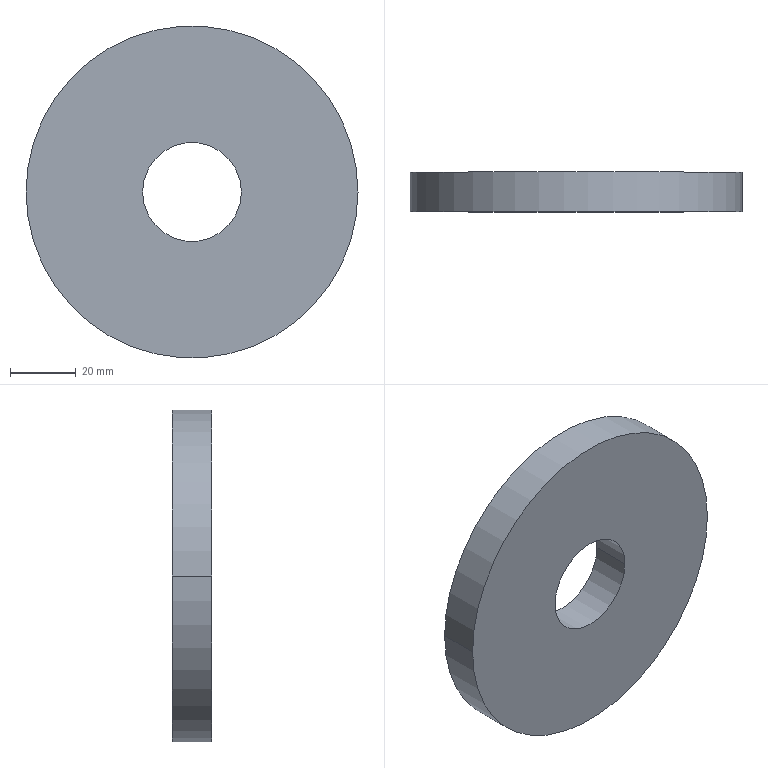Part | STEP file | ROLLER.4.stp | 1 solid | 6 faces | box 100.7 x 12 x 100.7 mm | volume 87081 mm3 | spline 6
STEP:
#1=CARTESIAN_POINT('',(0.,0.,0.));
#2=DIRECTION('',(0.,0.,1.));
#3=DIRECTION('',(1.,0.,0.));
#4=AXIS2_PLACEMENT_3D('',#1,#2,#3);
#5=CARTESIAN_POINT('',(15.,-6.,0.));
#6=VERTEX_POINT('',#5);
#7=CARTESIAN_POINT('',(-15.,-6.,0.));
#8=VERTEX_POINT('',#7);
#9=CARTESIAN_POINT('',(0.,-6.,0.));
#10=DIRECTION('',(0.,1.,0.));
#11=DIRECTION('',(1.,0.,0.));
#12=AXIS2_PLACEMENT_3D('',#9,#10,#11);
#13=CIRCLE('',#12,15.);
#14=CARTESIAN_POINT('',(50.35,-6.,-50.35));
#15=CARTESIAN_POINT('',(-50.35,-6.,-50.35));
#16=CARTESIAN_POINT('',(50.35,-6.,50.35));
#17=CARTESIAN_POINT('',(-50.35,-6.,50.35));
#18=B_SPLINE_SURFACE_WITH_KNOTS('',1,1,((#14,#15),(#16,#17)),.UNSPECIFIED.,.F.,.F.,.F.,(2,2),(2,2),(0.,100.7),(0.,100.7),.PIECEWISE_BEZIER_KNOTS.);
#19=CARTESIAN_POINT('',(50.35,35.35));
#20=CARTESIAN_POINT('',(49.636,35.349));
#21=CARTESIAN_POINT('',(48.208,35.452));
#22=CARTESIAN_POINT('',(46.11,35.909));
#23=CARTESIAN_POINT('',(44.098,36.659));
#24=CARTESIAN_POINT('',(42.213,37.688));
#25=CARTESIAN_POINT('',(40.494,38.975));
#26=CARTESIAN_POINT('',(38.975,40.494));
#27=CARTESIAN_POINT('',(37.688,42.213));
#28=CARTESIAN_POINT('',(36.659,44.098));
#29=CARTESIAN_POINT('',(35.909,46.11));
#30=CARTESIAN_POINT('',(35.452,48.208));
#31=CARTESIAN_POINT('',(35.299,50.35));
#32=CARTESIAN_POINT('',(35.452,52.492));
#33=CARTESIAN_POINT('',(35.909,54.59));
#34=CARTESIAN_POINT('',(36.659,56.602));
#35=CARTESIAN_POINT('',(37.688,58.487));
#36=CARTESIAN_POINT('',(38.975,60.206));
#37=CARTESIAN_POINT('',(40.494,61.725));
#38=CARTESIAN_POINT('',(42.213,63.012));
#39=CARTESIAN_POINT('',(44.098,64.041));
#40=CARTESIAN_POINT('',(46.11,64.791));
#41=CARTESIAN_POINT('',(48.208,65.248));
#42=CARTESIAN_POINT('',(49.636,65.351));
#43=CARTESIAN_POINT('',(50.35,65.35));
#44=B_SPLINE_CURVE_WITH_KNOTS('',3,(#19,#20,#21,#22,#23,#24,#25,#26,#27,#28,#29,#30,#31,#32,#33,#34,#35,#36,#37,#38,#39,#40,#41,#42,#43),.UNSPECIFIED.,.F.,.F.,(4,1,1,1,1,1,1,1,1,1,1,1,1,1,1,1,1,1,1,1,1,1,4),(0.,0.1428,0.2856,0.4284,0.5712,0.714,0.8568,0.9996,1.142,1.285,1.428,1.571,1.714,1.856,1.999,2.142,2.285,2.428,2.57,2.713,2.856,2.999,3.142),.QUASI_UNIFORM_KNOTS.);
#45=(GEOMETRIC_REPRESENTATION_CONTEXT(2)PARAMETRIC_REPRESENTATION_CONTEXT()REPRESENTATION_CONTEXT('',''));
#46=DEFINITIONAL_REPRESENTATION('',(#44),#45);
#47=PCURVE('',#18,#46);
#48=CARTESIAN_POINT('',(15.,-6.,0.));
#49=CARTESIAN_POINT('',(15.,-6.,-15.));
#50=CARTESIAN_POINT('',(0.,-6.,-15.));
#51=CARTESIAN_POINT('',(-15.,-6.,-15.));
#52=CARTESIAN_POINT('',(-15.,-6.,0.));
#53=CARTESIAN_POINT('',(15.,6.,0.));
#54=CARTESIAN_POINT('',(15.,6.,-15.));
#55=CARTESIAN_POINT('',(0.,6.,-15.));
#56=CARTESIAN_POINT('',(-15.,6.,-15.));
#57=CARTESIAN_POINT('',(-15.,6.,0.));
#58=(BOUNDED_SURFACE()B_SPLINE_SURFACE(1,2,((#48,#49,#50,#51,#52),(#53,#54,#55,#56,#57)),.UNSPECIFIED.,.F.,.F.,.F.)B_SPLINE_SURFACE_WITH_KNOTS((2,2),(3,2,3),(-0.4,0.4),(47.124,70.686,94.248),.UNSPECIFIED.)GEOMETRIC_REPRESENTATION_ITEM()RATIONAL_B_SPLINE_SURFACE(((1.,0.7071,1.,0.7071,1.),(1.,0.7071,1.,0.7071,1.)))REPRESENTATION_ITEM('')SURFACE());
#59=CARTESIAN_POINT('',(-0.4,47.124));
#60=CARTESIAN_POINT('',(-0.4,47.917));
#61=CARTESIAN_POINT('',(-0.4,49.457));
#62=CARTESIAN_POINT('',(-0.4,51.659));
#63=CARTESIAN_POINT('',(-0.4,53.782));
#64=CARTESIAN_POINT('',(-0.4,55.852));
#65=CARTESIAN_POINT('',(-0.4,57.891));
#66=CARTESIAN_POINT('',(-0.4,59.919));
#67=CARTESIAN_POINT('',(-0.4,61.958));
#68=CARTESIAN_POINT('',(-0.4,64.027));
#69=CARTESIAN_POINT('',(-0.4,66.153));
#70=CARTESIAN_POINT('',(-0.4,68.347));
#71=CARTESIAN_POINT('',(-0.4,70.686));
#72=CARTESIAN_POINT('',(-0.4,73.025));
#73=CARTESIAN_POINT('',(-0.4,75.219));
#74=CARTESIAN_POINT('',(-0.4,77.345));
#75=CARTESIAN_POINT('',(-0.4,79.414));
#76=CARTESIAN_POINT('',(-0.4,81.453));
#77=CARTESIAN_POINT('',(-0.4,83.481));
#78=CARTESIAN_POINT('',(-0.4,85.519));
#79=CARTESIAN_POINT('',(-0.4,87.589));
#80=CARTESIAN_POINT('',(-0.4,89.713));
#81=CARTESIAN_POINT('',(-0.4,91.915));
#82=CARTESIAN_POINT('',(-0.4,93.455));
#83=CARTESIAN_POINT('',(-0.4,94.248));
#84=B_SPLINE_CURVE_WITH_KNOTS('',3,(#59,#60,#61,#62,#63,#64,#65,#66,#67,#68,#69,#70,#71,#72,#73,#74,#75,#76,#77,#78,#79,#80,#81,#82,#83),.UNSPECIFIED.,.F.,.F.,(4,1,1,1,1,1,1,1,1,1,1,1,1,1,1,1,1,1,1,1,1,1,4),(0.,0.1428,0.2856,0.4284,0.5712,0.714,0.8568,0.9996,1.142,1.285,1.428,1.571,1.714,1.856,1.999,2.142,2.285,2.428,2.57,2.713,2.856,2.999,3.142),.QUASI_UNIFORM_KNOTS.);
#85=(GEOMETRIC_REPRESENTATION_CONTEXT(2)PARAMETRIC_REPRESENTATION_CONTEXT()REPRESENTATION_CONTEXT('',''));
#86=DEFINITIONAL_REPRESENTATION('',(#84),#85);
#87=PCURVE('',#58,#86);
#88=SURFACE_CURVE('',#13,(#47,#87),.PCURVE_S1.);
#89=EDGE_CURVE('',#6,#8,#88,.T.);
#90=ORIENTED_EDGE('',*,*,#89,.T.);
#91=CARTESIAN_POINT('',(0.,-6.,0.));
#92=DIRECTION('',(0.,1.,0.));
#93=DIRECTION('',(1.,0.,0.));
#94=AXIS2_PLACEMENT_3D('',#91,#92,#93);
#95=CIRCLE('',#94,15.);
#96=CARTESIAN_POINT('',(50.35,65.35));
#97=CARTESIAN_POINT('',(51.064,65.351));
#98=CARTESIAN_POINT('',(52.492,65.248));
#99=CARTESIAN_POINT('',(54.59,64.791));
#100=CARTESIAN_POINT('',(56.602,64.041));
#101=CARTESIAN_POINT('',(58.487,63.012));
#102=CARTESIAN_POINT('',(60.206,61.725));
#103=CARTESIAN_POINT('',(61.725,60.206));
#104=CARTESIAN_POINT('',(63.012,58.487));
#105=CARTESIAN_POINT('',(64.041,56.602));
#106=CARTESIAN_POINT('',(64.791,54.59));
#107=CARTESIAN_POINT('',(65.248,52.492));
#108=CARTESIAN_POINT('',(65.401,50.35));
#109=CARTESIAN_POINT('',(65.248,48.208));
#110=CARTESIAN_POINT('',(64.791,46.11));
#111=CARTESIAN_POINT('',(64.041,44.098));
#112=CARTESIAN_POINT('',(63.012,42.213));
#113=CARTESIAN_POINT('',(61.725,40.494));
#114=CARTESIAN_POINT('',(60.206,38.975));
#115=CARTESIAN_POINT('',(58.487,37.688));
#116=CARTESIAN_POINT('',(56.602,36.659));
#117=CARTESIAN_POINT('',(54.59,35.909));
#118=CARTESIAN_POINT('',(52.492,35.452));
#119=CARTESIAN_POINT('',(51.064,35.349));
#120=CARTESIAN_POINT('',(50.35,35.35));
#121=B_SPLINE_CURVE_WITH_KNOTS('',3,(#96,#97,#98,#99,#100,#101,#102,#103,#104,#105,#106,#107,#108,#109,#110,#111,#112,#113,#114,#115,#116,#117,#118,#119,#120),.UNSPECIFIED.,.F.,.F.,(4,1,1,1,1,1,1,1,1,1,1,1,1,1,1,1,1,1,1,1,1,1,4),(3.142,3.284,3.427,3.57,3.713,3.856,3.998,4.141,4.284,4.427,4.57,4.712,4.855,4.998,5.141,5.284,5.426,5.569,5.712,5.855,5.998,6.14,6.283),.QUASI_UNIFORM_KNOTS.);
#122=(GEOMETRIC_REPRESENTATION_CONTEXT(2)PARAMETRIC_REPRESENTATION_CONTEXT()REPRESENTATION_CONTEXT('',''));
#123=DEFINITIONAL_REPRESENTATION('',(#121),#122);
#124=PCURVE('',#18,#123);
#125=CARTESIAN_POINT('',(-15.,-6.,0.));
#126=CARTESIAN_POINT('',(-15.,-6.,15.));
#127=CARTESIAN_POINT('',(0.,-6.,15.));
#128=CARTESIAN_POINT('',(15.,-6.,15.));
#129=CARTESIAN_POINT('',(15.,-6.,0.));
#130=CARTESIAN_POINT('',(-15.,6.,0.));
#131=CARTESIAN_POINT('',(-15.,6.,15.));
#132=CARTESIAN_POINT('',(0.,6.,15.));
#133=CARTESIAN_POINT('',(15.,6.,15.));
#134=CARTESIAN_POINT('',(15.,6.,0.));
#135=(BOUNDED_SURFACE()B_SPLINE_SURFACE(1,2,((#125,#126,#127,#128,#129),(#130,#131,#132,#133,#134)),.UNSPECIFIED.,.F.,.F.,.F.)B_SPLINE_SURFACE_WITH_KNOTS((2,2),(3,2,3),(-0.4,0.4),(0.,23.562,47.124),.PIECEWISE_BEZIER_KNOTS.)GEOMETRIC_REPRESENTATION_ITEM()RATIONAL_B_SPLINE_SURFACE(((1.,0.7071,1.,0.7071,1.),(1.,0.7071,1.,0.7071,1.)))REPRESENTATION_ITEM('')SURFACE());
#136=CARTESIAN_POINT('',(-0.4,0.));
#137=CARTESIAN_POINT('',(-0.4,0.7927));
#138=CARTESIAN_POINT('',(-0.4,2.333));
#139=CARTESIAN_POINT('',(-0.4,4.535));
#140=CARTESIAN_POINT('',(-0.4,6.658));
#141=CARTESIAN_POINT('',(-0.4,8.728));
#142=CARTESIAN_POINT('',(-0.4,10.767));
#143=CARTESIAN_POINT('',(-0.4,12.795));
#144=CARTESIAN_POINT('',(-0.4,14.834));
#145=CARTESIAN_POINT('',(-0.4,16.903));
#146=CARTESIAN_POINT('',(-0.4,19.029));
#147=CARTESIAN_POINT('',(-0.4,21.223));
#148=CARTESIAN_POINT('',(-0.4,23.562));
#149=CARTESIAN_POINT('',(-0.4,25.901));
#150=CARTESIAN_POINT('',(-0.4,28.095));
#151=CARTESIAN_POINT('',(-0.4,30.221));
#152=CARTESIAN_POINT('',(-0.4,32.29));
#153=CARTESIAN_POINT('',(-0.4,34.329));
#154=CARTESIAN_POINT('',(-0.4,36.357));
#155=CARTESIAN_POINT('',(-0.4,38.395));
#156=CARTESIAN_POINT('',(-0.4,40.465));
#157=CARTESIAN_POINT('',(-0.4,42.589));
#158=CARTESIAN_POINT('',(-0.4,44.791));
#159=CARTESIAN_POINT('',(-0.4,46.331));
#160=CARTESIAN_POINT('',(-0.4,47.124));
#161=B_SPLINE_CURVE_WITH_KNOTS('',3,(#136,#137,#138,#139,#140,#141,#142,#143,#144,#145,#146,#147,#148,#149,#150,#151,#152,#153,#154,#155,#156,#157,#158,#159,#160),.UNSPECIFIED.,.F.,.F.,(4,1,1,1,1,1,1,1,1,1,1,1,1,1,1,1,1,1,1,1,1,1,4),(3.142,3.284,3.427,3.57,3.713,3.856,3.998,4.141,4.284,4.427,4.57,4.712,4.855,4.998,5.141,5.284,5.426,5.569,5.712,5.855,5.998,6.14,6.283),.QUASI_UNIFORM_KNOTS.);
#162=(GEOMETRIC_REPRESENTATION_CONTEXT(2)PARAMETRIC_REPRESENTATION_CONTEXT()REPRESENTATION_CONTEXT('',''));
#163=DEFINITIONAL_REPRESENTATION('',(#161),#162);
#164=PCURVE('',#135,#163);
#165=SURFACE_CURVE('',#95,(#124,#164),.PCURVE_S1.);
#166=EDGE_CURVE('',#8,#6,#165,.T.);
#167=ORIENTED_EDGE('',*,*,#166,.T.);
#168=EDGE_LOOP('',(#90,#167));
#169=FACE_BOUND('',#168,.T.);
#170=CARTESIAN_POINT('',(50.35,-6.,0.));
#171=VERTEX_POINT('',#170);
#172=CARTESIAN_POINT('',(-50.35,-6.,0.));
#173=VERTEX_POINT('',#172);
#174=CARTESIAN_POINT('',(0.,-6.,0.));
#175=DIRECTION('',(0.,1.,0.));
#176=DIRECTION('',(1.,0.,0.));
#177=AXIS2_PLACEMENT_3D('',#174,#175,#176);
#178=CIRCLE('',#177,50.35);
#179=CARTESIAN_POINT('',(50.35,0.));
#180=CARTESIAN_POINT('',(47.953,-0.001715));
#181=CARTESIAN_POINT('',(43.16,0.3436));
#182=CARTESIAN_POINT('',(36.116,1.875));
#183=CARTESIAN_POINT('',(29.363,4.394));
#184=CARTESIAN_POINT('',(23.036,7.849));
#185=CARTESIAN_POINT('',(17.266,12.168));
#186=CARTESIAN_POINT('',(12.168,17.266));
#187=CARTESIAN_POINT('',(7.849,23.036));
#188=CARTESIAN_POINT('',(4.394,29.363));
#189=CARTESIAN_POINT('',(1.875,36.116));
#190=CARTESIAN_POINT('',(0.3428,43.16));
#191=CARTESIAN_POINT('',(-0.1714,50.35));
#192=CARTESIAN_POINT('',(0.3428,57.54));
#193=CARTESIAN_POINT('',(1.875,64.584));
#194=CARTESIAN_POINT('',(4.394,71.337));
#195=CARTESIAN_POINT('',(7.849,77.664));
#196=CARTESIAN_POINT('',(12.168,83.434));
#197=CARTESIAN_POINT('',(17.266,88.532));
#198=CARTESIAN_POINT('',(23.036,92.851));
#199=CARTESIAN_POINT('',(29.363,96.306));
#200=CARTESIAN_POINT('',(36.116,98.825));
#201=CARTESIAN_POINT('',(43.16,100.356));
#202=CARTESIAN_POINT('',(47.953,100.702));
#203=CARTESIAN_POINT('',(50.35,100.7));
#204=B_SPLINE_CURVE_WITH_KNOTS('',3,(#179,#180,#181,#182,#183,#184,#185,#186,#187,#188,#189,#190,#191,#192,#193,#194,#195,#196,#197,#198,#199,#200,#201,#202,#203),.UNSPECIFIED.,.F.,.F.,(4,1,1,1,1,1,1,1,1,1,1,1,1,1,1,1,1,1,1,1,1,1,4),(0.,0.1428,0.2856,0.4284,0.5712,0.714,0.8568,0.9996,1.142,1.285,1.428,1.571,1.714,1.856,1.999,2.142,2.285,2.428,2.57,2.713,2.856,2.999,3.142),.QUASI_UNIFORM_KNOTS.);
#205=(GEOMETRIC_REPRESENTATION_CONTEXT(2)PARAMETRIC_REPRESENTATION_CONTEXT()REPRESENTATION_CONTEXT('',''));
#206=DEFINITIONAL_REPRESENTATION('',(#204),#205);
#207=PCURVE('',#18,#206);
#208=CARTESIAN_POINT('',(50.35,6.,0.));
#209=CARTESIAN_POINT('',(50.35,6.,-50.35));
#210=CARTESIAN_POINT('',(0.,6.,-50.35));
#211=CARTESIAN_POINT('',(-50.35,6.,-50.35));
#212=CARTESIAN_POINT('',(-50.35,6.,0.));
#213=CARTESIAN_POINT('',(50.35,-6.,0.));
#214=CARTESIAN_POINT('',(50.35,-6.,-50.35));
#215=CARTESIAN_POINT('',(0.,-6.,-50.35));
#216=CARTESIAN_POINT('',(-50.35,-6.,-50.35));
#217=CARTESIAN_POINT('',(-50.35,-6.,0.));
#218=(BOUNDED_SURFACE()B_SPLINE_SURFACE(1,2,((#208,#209,#210,#211,#212),(#213,#214,#215,#216,#217)),.UNSPECIFIED.,.F.,.F.,.F.)B_SPLINE_SURFACE_WITH_KNOTS((2,2),(3,2,3),(-0.1192,0.1192),(158.179,237.269,316.358),.PIECEWISE_BEZIER_KNOTS.)GEOMETRIC_REPRESENTATION_ITEM()RATIONAL_B_SPLINE_SURFACE(((1.,0.7071,1.,0.7071,1.),(1.,0.7071,1.,0.7071,1.)))REPRESENTATION_ITEM('')SURFACE());
#219=CARTESIAN_POINT('',(0.1192,158.179));
#220=CARTESIAN_POINT('',(0.1192,160.84));
#221=CARTESIAN_POINT('',(0.1192,166.009));
#222=CARTESIAN_POINT('',(0.1192,173.401));
#223=CARTESIAN_POINT('',(0.1192,180.53));
#224=CARTESIAN_POINT('',(0.1192,187.478));
#225=CARTESIAN_POINT('',(0.1192,194.32));
#226=CARTESIAN_POINT('',(0.1192,201.128));
#227=CARTESIAN_POINT('',(0.1192,207.971));
#228=CARTESIAN_POINT('',(0.1192,214.917));
#229=CARTESIAN_POINT('',(0.1192,222.053));
#230=CARTESIAN_POINT('',(0.1192,229.419));
#231=CARTESIAN_POINT('',(0.1192,237.269));
#232=CARTESIAN_POINT('',(0.1192,245.119));
#233=CARTESIAN_POINT('',(0.1192,252.485));
#234=CARTESIAN_POINT('',(0.1192,259.621));
#235=CARTESIAN_POINT('',(0.1192,266.567));
#236=CARTESIAN_POINT('',(0.1192,273.41));
#237=CARTESIAN_POINT('',(0.1192,280.217));
#238=CARTESIAN_POINT('',(0.1192,287.06));
#239=CARTESIAN_POINT('',(0.1192,294.008));
#240=CARTESIAN_POINT('',(0.1192,301.137));
#241=CARTESIAN_POINT('',(0.1192,308.529));
#242=CARTESIAN_POINT('',(0.1192,313.698));
#243=CARTESIAN_POINT('',(0.1192,316.358));
#244=B_SPLINE_CURVE_WITH_KNOTS('',3,(#219,#220,#221,#222,#223,#224,#225,#226,#227,#228,#229,#230,#231,#232,#233,#234,#235,#236,#237,#238,#239,#240,#241,#242,#243),.UNSPECIFIED.,.F.,.F.,(4,1,1,1,1,1,1,1,1,1,1,1,1,1,1,1,1,1,1,1,1,1,4),(0.,0.1428,0.2856,0.4284,0.5712,0.714,0.8568,0.9996,1.142,1.285,1.428,1.571,1.714,1.856,1.999,2.142,2.285,2.428,2.57,2.713,2.856,2.999,3.142),.QUASI_UNIFORM_KNOTS.);
#245=(GEOMETRIC_REPRESENTATION_CONTEXT(2)PARAMETRIC_REPRESENTATION_CONTEXT()REPRESENTATION_CONTEXT('',''));
#246=DEFINITIONAL_REPRESENTATION('',(#244),#245);
#247=PCURVE('',#218,#246);
#248=SURFACE_CURVE('',#178,(#207,#247),.PCURVE_S1.);
#249=EDGE_CURVE('',#171,#173,#248,.T.);
#250=ORIENTED_EDGE('',*,*,#249,.F.);
#251=CARTESIAN_POINT('',(0.,-6.,0.));
#252=DIRECTION('',(0.,1.,0.));
#253=DIRECTION('',(1.,0.,0.));
#254=AXIS2_PLACEMENT_3D('',#251,#252,#253);
#255=CIRCLE('',#254,50.35);
#256=CARTESIAN_POINT('',(50.35,100.7));
#257=CARTESIAN_POINT('',(52.747,100.702));
#258=CARTESIAN_POINT('',(57.54,100.356));
#259=CARTESIAN_POINT('',(64.584,98.825));
#260=CARTESIAN_POINT('',(71.337,96.306));
#261=CARTESIAN_POINT('',(77.664,92.851));
#262=CARTESIAN_POINT('',(83.434,88.532));
#263=CARTESIAN_POINT('',(88.532,83.434));
#264=CARTESIAN_POINT('',(92.851,77.664));
#265=CARTESIAN_POINT('',(96.306,71.337));
#266=CARTESIAN_POINT('',(98.825,64.584));
#267=CARTESIAN_POINT('',(100.357,57.54));
#268=CARTESIAN_POINT('',(100.871,50.35));
#269=CARTESIAN_POINT('',(100.357,43.16));
#270=CARTESIAN_POINT('',(98.825,36.116));
#271=CARTESIAN_POINT('',(96.306,29.363));
#272=CARTESIAN_POINT('',(92.851,23.036));
#273=CARTESIAN_POINT('',(88.532,17.266));
#274=CARTESIAN_POINT('',(83.434,12.168));
#275=CARTESIAN_POINT('',(77.664,7.849));
#276=CARTESIAN_POINT('',(71.337,4.394));
#277=CARTESIAN_POINT('',(64.584,1.875));
#278=CARTESIAN_POINT('',(57.54,0.3436));
#279=CARTESIAN_POINT('',(52.747,-0.001715));
#280=CARTESIAN_POINT('',(50.35,0.));
#281=B_SPLINE_CURVE_WITH_KNOTS('',3,(#256,#257,#258,#259,#260,#261,#262,#263,#264,#265,#266,#267,#268,#269,#270,#271,#272,#273,#274,#275,#276,#277,#278,#279,#280),.UNSPECIFIED.,.F.,.F.,(4,1,1,1,1,1,1,1,1,1,1,1,1,1,1,1,1,1,1,1,1,1,4),(3.142,3.284,3.427,3.57,3.713,3.856,3.998,4.141,4.284,4.427,4.57,4.712,4.855,4.998,5.141,5.284,5.426,5.569,5.712,5.855,5.998,6.14,6.283),.QUASI_UNIFORM_KNOTS.);
#282=(GEOMETRIC_REPRESENTATION_CONTEXT(2)PARAMETRIC_REPRESENTATION_CONTEXT()REPRESENTATION_CONTEXT('',''));
#283=DEFINITIONAL_REPRESENTATION('',(#281),#282);
#284=PCURVE('',#18,#283);
#285=CARTESIAN_POINT('',(-50.35,6.,0.));
#286=CARTESIAN_POINT('',(-50.35,6.,50.35));
#287=CARTESIAN_POINT('',(0.,6.,50.35));
#288=CARTESIAN_POINT('',(50.35,6.,50.35));
#289=CARTESIAN_POINT('',(50.35,6.,0.));
#290=CARTESIAN_POINT('',(-50.35,-6.,0.));
#291=CARTESIAN_POINT('',(-50.35,-6.,50.35));
#292=CARTESIAN_POINT('',(0.,-6.,50.35));
#293=CARTESIAN_POINT('',(50.35,-6.,50.35));
#294=CARTESIAN_POINT('',(50.35,-6.,0.));
#295=(BOUNDED_SURFACE()B_SPLINE_SURFACE(1,2,((#285,#286,#287,#288,#289),(#290,#291,#292,#293,#294)),.UNSPECIFIED.,.F.,.F.,.F.)B_SPLINE_SURFACE_WITH_KNOTS((2,2),(3,2,3),(-0.1192,0.1192),(0.,79.09,158.179),.UNSPECIFIED.)GEOMETRIC_REPRESENTATION_ITEM()RATIONAL_B_SPLINE_SURFACE(((1.,0.7071,1.,0.7071,1.),(1.,0.7071,1.,0.7071,1.)))REPRESENTATION_ITEM('')SURFACE());
#296=CARTESIAN_POINT('',(0.1192,0.));
#297=CARTESIAN_POINT('',(0.1192,2.661));
#298=CARTESIAN_POINT('',(0.1192,7.83));
#299=CARTESIAN_POINT('',(0.1192,15.221));
#300=CARTESIAN_POINT('',(0.1192,22.35));
#301=CARTESIAN_POINT('',(0.1192,29.298));
#302=CARTESIAN_POINT('',(0.1192,36.141));
#303=CARTESIAN_POINT('',(0.1192,42.949));
#304=CARTESIAN_POINT('',(0.1192,49.792));
#305=CARTESIAN_POINT('',(0.1192,56.738));
#306=CARTESIAN_POINT('',(0.1192,63.874));
#307=CARTESIAN_POINT('',(0.1192,71.239));
#308=CARTESIAN_POINT('',(0.1192,79.09));
#309=CARTESIAN_POINT('',(0.1192,86.94));
#310=CARTESIAN_POINT('',(0.1192,94.306));
#311=CARTESIAN_POINT('',(0.1192,101.441));
#312=CARTESIAN_POINT('',(0.1192,108.388));
#313=CARTESIAN_POINT('',(0.1192,115.231));
#314=CARTESIAN_POINT('',(0.1192,122.038));
#315=CARTESIAN_POINT('',(0.1192,128.881));
#316=CARTESIAN_POINT('',(0.1192,135.829));
#317=CARTESIAN_POINT('',(0.1192,142.958));
#318=CARTESIAN_POINT('',(0.1192,150.349));
#319=CARTESIAN_POINT('',(0.1192,155.519));
#320=CARTESIAN_POINT('',(0.1192,158.179));
#321=B_SPLINE_CURVE_WITH_KNOTS('',3,(#296,#297,#298,#299,#300,#301,#302,#303,#304,#305,#306,#307,#308,#309,#310,#311,#312,#313,#314,#315,#316,#317,#318,#319,#320),.UNSPECIFIED.,.F.,.F.,(4,1,1,1,1,1,1,1,1,1,1,1,1,1,1,1,1,1,1,1,1,1,4),(3.142,3.284,3.427,3.57,3.713,3.856,3.998,4.141,4.284,4.427,4.57,4.712,4.855,4.998,5.141,5.284,5.426,5.569,5.712,5.855,5.998,6.14,6.283),.QUASI_UNIFORM_KNOTS.);
#322=(GEOMETRIC_REPRESENTATION_CONTEXT(2)PARAMETRIC_REPRESENTATION_CONTEXT()REPRESENTATION_CONTEXT('',''));
#323=DEFINITIONAL_REPRESENTATION('',(#321),#322);
#324=PCURVE('',#295,#323);
#325=SURFACE_CURVE('',#255,(#284,#324),.PCURVE_S1.);
#326=EDGE_CURVE('',#173,#171,#325,.T.);
#327=ORIENTED_EDGE('',*,*,#326,.F.);
#328=EDGE_LOOP('',(#250,#327));
#329=FACE_BOUND('',#328,.T.);
#330=ADVANCED_FACE('',(#169,#329),#18,.T.);
#331=CARTESIAN_POINT('',(50.35,6.,0.));
#332=VERTEX_POINT('',#331);
#333=CARTESIAN_POINT('',(50.35,-6.,0.));
#334=DIRECTION('',(0.,1.,0.));
#335=VECTOR('',#334,1.);
#336=LINE('',#333,#335);
#337=CARTESIAN_POINT('',(0.1192,158.179));
#338=CARTESIAN_POINT('',(-0.1192,158.179));
#339=B_SPLINE_CURVE_WITH_KNOTS('',1,(#337,#338),.UNSPECIFIED.,.F.,.F.,(2,2),(0.,12.),.PIECEWISE_BEZIER_KNOTS.);
#340=(GEOMETRIC_REPRESENTATION_CONTEXT(2)PARAMETRIC_REPRESENTATION_CONTEXT()REPRESENTATION_CONTEXT('',''));
#341=DEFINITIONAL_REPRESENTATION('',(#339),#340);
#342=PCURVE('',#295,#341);
#343=CARTESIAN_POINT('',(0.1192,158.179));
#344=CARTESIAN_POINT('',(-0.1192,158.179));
#345=B_SPLINE_CURVE_WITH_KNOTS('',1,(#343,#344),.UNSPECIFIED.,.F.,.F.,(2,2),(0.,12.),.PIECEWISE_BEZIER_KNOTS.);
#346=(GEOMETRIC_REPRESENTATION_CONTEXT(2)PARAMETRIC_REPRESENTATION_CONTEXT()REPRESENTATION_CONTEXT('',''));
#347=DEFINITIONAL_REPRESENTATION('',(#345),#346);
#348=PCURVE('',#218,#347);
#349=SURFACE_CURVE('',#336,(#342,#348),.PCURVE_S1.);
#350=EDGE_CURVE('',#171,#332,#349,.T.);
#351=ORIENTED_EDGE('',*,*,#350,.T.);
#352=CARTESIAN_POINT('',(-50.35,6.,0.));
#353=VERTEX_POINT('',#352);
#354=CARTESIAN_POINT('',(0.,6.,0.));
#355=DIRECTION('',(0.,1.,0.));
#356=DIRECTION('',(1.,0.,0.));
#357=AXIS2_PLACEMENT_3D('',#354,#355,#356);
#358=CIRCLE('',#357,50.35);
#359=CARTESIAN_POINT('',(-0.1192,0.));
#360=CARTESIAN_POINT('',(-0.1192,2.661));
#361=CARTESIAN_POINT('',(-0.1192,7.83));
#362=CARTESIAN_POINT('',(-0.1192,15.221));
#363=CARTESIAN_POINT('',(-0.1192,22.35));
#364=CARTESIAN_POINT('',(-0.1192,29.298));
#365=CARTESIAN_POINT('',(-0.1192,36.141));
#366=CARTESIAN_POINT('',(-0.1192,42.949));
#367=CARTESIAN_POINT('',(-0.1192,49.792));
#368=CARTESIAN_POINT('',(-0.1192,56.738));
#369=CARTESIAN_POINT('',(-0.1192,63.874));
#370=CARTESIAN_POINT('',(-0.1192,71.239));
#371=CARTESIAN_POINT('',(-0.1192,79.09));
#372=CARTESIAN_POINT('',(-0.1192,86.94));
#373=CARTESIAN_POINT('',(-0.1192,94.306));
#374=CARTESIAN_POINT('',(-0.1192,101.441));
#375=CARTESIAN_POINT('',(-0.1192,108.388));
#376=CARTESIAN_POINT('',(-0.1192,115.231));
#377=CARTESIAN_POINT('',(-0.1192,122.038));
#378=CARTESIAN_POINT('',(-0.1192,128.881));
#379=CARTESIAN_POINT('',(-0.1192,135.829));
#380=CARTESIAN_POINT('',(-0.1192,142.958));
#381=CARTESIAN_POINT('',(-0.1192,150.349));
#382=CARTESIAN_POINT('',(-0.1192,155.519));
#383=CARTESIAN_POINT('',(-0.1192,158.179));
#384=B_SPLINE_CURVE_WITH_KNOTS('',3,(#359,#360,#361,#362,#363,#364,#365,#366,#367,#368,#369,#370,#371,#372,#373,#374,#375,#376,#377,#378,#379,#380,#381,#382,#383),.UNSPECIFIED.,.F.,.F.,(4,1,1,1,1,1,1,1,1,1,1,1,1,1,1,1,1,1,1,1,1,1,4),(3.142,3.284,3.427,3.57,3.713,3.856,3.998,4.141,4.284,4.427,4.57,4.712,4.855,4.998,5.141,5.284,5.426,5.569,5.712,5.855,5.998,6.14,6.283),.QUASI_UNIFORM_KNOTS.);
#385=(GEOMETRIC_REPRESENTATION_CONTEXT(2)PARAMETRIC_REPRESENTATION_CONTEXT()REPRESENTATION_CONTEXT('',''));
#386=DEFINITIONAL_REPRESENTATION('',(#384),#385);
#387=PCURVE('',#295,#386);
#388=CARTESIAN_POINT('',(50.35,6.,50.35));
#389=CARTESIAN_POINT('',(-50.35,6.,50.35));
#390=CARTESIAN_POINT('',(50.35,6.,-50.35));
#391=CARTESIAN_POINT('',(-50.35,6.,-50.35));
#392=B_SPLINE_SURFACE_WITH_KNOTS('',1,1,((#388,#389),(#390,#391)),.UNSPECIFIED.,.F.,.F.,.F.,(2,2),(2,2),(0.,100.7),(0.,100.7),.PIECEWISE_BEZIER_KNOTS.);
#393=CARTESIAN_POINT('',(50.35,100.7));
#394=CARTESIAN_POINT('',(47.953,100.702));
#395=CARTESIAN_POINT('',(43.16,100.356));
#396=CARTESIAN_POINT('',(36.116,98.825));
#397=CARTESIAN_POINT('',(29.363,96.306));
#398=CARTESIAN_POINT('',(23.036,92.851));
#399=CARTESIAN_POINT('',(17.266,88.532));
#400=CARTESIAN_POINT('',(12.168,83.434));
#401=CARTESIAN_POINT('',(7.849,77.664));
#402=CARTESIAN_POINT('',(4.394,71.337));
#403=CARTESIAN_POINT('',(1.875,64.584));
#404=CARTESIAN_POINT('',(0.3428,57.54));
#405=CARTESIAN_POINT('',(-0.1714,50.35));
#406=CARTESIAN_POINT('',(0.3428,43.16));
#407=CARTESIAN_POINT('',(1.875,36.116));
#408=CARTESIAN_POINT('',(4.394,29.363));
#409=CARTESIAN_POINT('',(7.849,23.036));
#410=CARTESIAN_POINT('',(12.168,17.266));
#411=CARTESIAN_POINT('',(17.266,12.168));
#412=CARTESIAN_POINT('',(23.036,7.849));
#413=CARTESIAN_POINT('',(29.363,4.394));
#414=CARTESIAN_POINT('',(36.116,1.875));
#415=CARTESIAN_POINT('',(43.16,0.3436));
#416=CARTESIAN_POINT('',(47.953,-0.001715));
#417=CARTESIAN_POINT('',(50.35,0.));
#418=B_SPLINE_CURVE_WITH_KNOTS('',3,(#393,#394,#395,#396,#397,#398,#399,#400,#401,#402,#403,#404,#405,#406,#407,#408,#409,#410,#411,#412,#413,#414,#415,#416,#417),.UNSPECIFIED.,.F.,.F.,(4,1,1,1,1,1,1,1,1,1,1,1,1,1,1,1,1,1,1,1,1,1,4),(3.142,3.284,3.427,3.57,3.713,3.856,3.998,4.141,4.284,4.427,4.57,4.712,4.855,4.998,5.141,5.284,5.426,5.569,5.712,5.855,5.998,6.14,6.283),.QUASI_UNIFORM_KNOTS.);
#419=(GEOMETRIC_REPRESENTATION_CONTEXT(2)PARAMETRIC_REPRESENTATION_CONTEXT()REPRESENTATION_CONTEXT('',''));
#420=DEFINITIONAL_REPRESENTATION('',(#418),#419);
#421=PCURVE('',#392,#420);
#422=SURFACE_CURVE('',#358,(#387,#421),.PCURVE_S1.);
#423=EDGE_CURVE('',#353,#332,#422,.T.);
#424=ORIENTED_EDGE('',*,*,#423,.F.);
#425=CARTESIAN_POINT('',(-50.35,-6.,0.));
#426=DIRECTION('',(0.,1.,0.));
#427=VECTOR('',#426,1.);
#428=LINE('',#425,#427);
#429=CARTESIAN_POINT('',(0.1192,0.));
#430=CARTESIAN_POINT('',(-0.1192,0.));
#431=B_SPLINE_CURVE_WITH_KNOTS('',1,(#429,#430),.UNSPECIFIED.,.F.,.F.,(2,2),(0.,12.),.PIECEWISE_BEZIER_KNOTS.);
#432=(GEOMETRIC_REPRESENTATION_CONTEXT(2)PARAMETRIC_REPRESENTATION_CONTEXT()REPRESENTATION_CONTEXT('',''));
#433=DEFINITIONAL_REPRESENTATION('',(#431),#432);
#434=PCURVE('',#295,#433);
#435=CARTESIAN_POINT('',(0.1192,316.358));
#436=CARTESIAN_POINT('',(-0.1192,316.358));
#437=B_SPLINE_CURVE_WITH_KNOTS('',1,(#435,#436),.UNSPECIFIED.,.F.,.F.,(2,2),(0.,12.),.PIECEWISE_BEZIER_KNOTS.);
#438=(GEOMETRIC_REPRESENTATION_CONTEXT(2)PARAMETRIC_REPRESENTATION_CONTEXT()REPRESENTATION_CONTEXT('',''));
#439=DEFINITIONAL_REPRESENTATION('',(#437),#438);
#440=PCURVE('',#218,#439);
#441=SURFACE_CURVE('',#428,(#434,#440),.PCURVE_S1.);
#442=EDGE_CURVE('',#173,#353,#441,.T.);
#443=ORIENTED_EDGE('',*,*,#442,.F.);
#444=ORIENTED_EDGE('',*,*,#326,.T.);
#445=EDGE_LOOP('',(#351,#424,#443,#444));
#446=FACE_BOUND('',#445,.T.);
#447=ADVANCED_FACE('',(#446),#295,.T.);
#448=CARTESIAN_POINT('',(15.,6.,0.));
#449=VERTEX_POINT('',#448);
#450=CARTESIAN_POINT('',(-15.,6.,0.));
#451=VERTEX_POINT('',#450);
#452=CARTESIAN_POINT('',(0.,6.,0.));
#453=DIRECTION('',(0.,1.,0.));
#454=DIRECTION('',(1.,0.,0.));
#455=AXIS2_PLACEMENT_3D('',#452,#453,#454);
#456=CIRCLE('',#455,15.);
#457=CARTESIAN_POINT('',(50.35,35.35));
#458=CARTESIAN_POINT('',(51.064,35.349));
#459=CARTESIAN_POINT('',(52.492,35.452));
#460=CARTESIAN_POINT('',(54.59,35.909));
#461=CARTESIAN_POINT('',(56.602,36.659));
#462=CARTESIAN_POINT('',(58.487,37.688));
#463=CARTESIAN_POINT('',(60.206,38.975));
#464=CARTESIAN_POINT('',(61.725,40.494));
#465=CARTESIAN_POINT('',(63.012,42.213));
#466=CARTESIAN_POINT('',(64.041,44.098));
#467=CARTESIAN_POINT('',(64.791,46.11));
#468=CARTESIAN_POINT('',(65.248,48.208));
#469=CARTESIAN_POINT('',(65.401,50.35));
#470=CARTESIAN_POINT('',(65.248,52.492));
#471=CARTESIAN_POINT('',(64.791,54.59));
#472=CARTESIAN_POINT('',(64.041,56.602));
#473=CARTESIAN_POINT('',(63.012,58.487));
#474=CARTESIAN_POINT('',(61.725,60.206));
#475=CARTESIAN_POINT('',(60.206,61.725));
#476=CARTESIAN_POINT('',(58.487,63.012));
#477=CARTESIAN_POINT('',(56.602,64.041));
#478=CARTESIAN_POINT('',(54.59,64.791));
#479=CARTESIAN_POINT('',(52.492,65.248));
#480=CARTESIAN_POINT('',(51.064,65.351));
#481=CARTESIAN_POINT('',(50.35,65.35));
#482=B_SPLINE_CURVE_WITH_KNOTS('',3,(#457,#458,#459,#460,#461,#462,#463,#464,#465,#466,#467,#468,#469,#470,#471,#472,#473,#474,#475,#476,#477,#478,#479,#480,#481),.UNSPECIFIED.,.F.,.F.,(4,1,1,1,1,1,1,1,1,1,1,1,1,1,1,1,1,1,1,1,1,1,4),(0.,0.1428,0.2856,0.4284,0.5712,0.714,0.8568,0.9996,1.142,1.285,1.428,1.571,1.714,1.856,1.999,2.142,2.285,2.428,2.57,2.713,2.856,2.999,3.142),.QUASI_UNIFORM_KNOTS.);
#483=(GEOMETRIC_REPRESENTATION_CONTEXT(2)PARAMETRIC_REPRESENTATION_CONTEXT()REPRESENTATION_CONTEXT('',''));
#484=DEFINITIONAL_REPRESENTATION('',(#482),#483);
#485=PCURVE('',#392,#484);
#486=CARTESIAN_POINT('',(0.4,47.124));
#487=CARTESIAN_POINT('',(0.4,47.917));
#488=CARTESIAN_POINT('',(0.4,49.457));
#489=CARTESIAN_POINT('',(0.4,51.659));
#490=CARTESIAN_POINT('',(0.4,53.782));
#491=CARTESIAN_POINT('',(0.4,55.852));
#492=CARTESIAN_POINT('',(0.4,57.891));
#493=CARTESIAN_POINT('',(0.4,59.919));
#494=CARTESIAN_POINT('',(0.4,61.958));
#495=CARTESIAN_POINT('',(0.4,64.027));
#496=CARTESIAN_POINT('',(0.4,66.153));
#497=CARTESIAN_POINT('',(0.4,68.347));
#498=CARTESIAN_POINT('',(0.4,70.686));
#499=CARTESIAN_POINT('',(0.4,73.025));
#500=CARTESIAN_POINT('',(0.4,75.219));
#501=CARTESIAN_POINT('',(0.4,77.345));
#502=CARTESIAN_POINT('',(0.4,79.414));
#503=CARTESIAN_POINT('',(0.4,81.453));
#504=CARTESIAN_POINT('',(0.4,83.481));
#505=CARTESIAN_POINT('',(0.4,85.519));
#506=CARTESIAN_POINT('',(0.4,87.589));
#507=CARTESIAN_POINT('',(0.4,89.713));
#508=CARTESIAN_POINT('',(0.4,91.915));
#509=CARTESIAN_POINT('',(0.4,93.455));
#510=CARTESIAN_POINT('',(0.4,94.248));
#511=B_SPLINE_CURVE_WITH_KNOTS('',3,(#486,#487,#488,#489,#490,#491,#492,#493,#494,#495,#496,#497,#498,#499,#500,#501,#502,#503,#504,#505,#506,#507,#508,#509,#510),.UNSPECIFIED.,.F.,.F.,(4,1,1,1,1,1,1,1,1,1,1,1,1,1,1,1,1,1,1,1,1,1,4),(0.,0.1428,0.2856,0.4284,0.5712,0.714,0.8568,0.9996,1.142,1.285,1.428,1.571,1.714,1.856,1.999,2.142,2.285,2.428,2.57,2.713,2.856,2.999,3.142),.QUASI_UNIFORM_KNOTS.);
#512=(GEOMETRIC_REPRESENTATION_CONTEXT(2)PARAMETRIC_REPRESENTATION_CONTEXT()REPRESENTATION_CONTEXT('',''));
#513=DEFINITIONAL_REPRESENTATION('',(#511),#512);
#514=PCURVE('',#58,#513);
#515=SURFACE_CURVE('',#456,(#485,#514),.PCURVE_S1.);
#516=EDGE_CURVE('',#449,#451,#515,.T.);
#517=ORIENTED_EDGE('',*,*,#516,.F.);
#518=CARTESIAN_POINT('',(0.,6.,0.));
#519=DIRECTION('',(0.,1.,0.));
#520=DIRECTION('',(1.,0.,0.));
#521=AXIS2_PLACEMENT_3D('',#518,#519,#520);
#522=CIRCLE('',#521,15.);
#523=CARTESIAN_POINT('',(50.35,65.35));
#524=CARTESIAN_POINT('',(49.636,65.351));
#525=CARTESIAN_POINT('',(48.208,65.248));
#526=CARTESIAN_POINT('',(46.11,64.791));
#527=CARTESIAN_POINT('',(44.098,64.041));
#528=CARTESIAN_POINT('',(42.213,63.012));
#529=CARTESIAN_POINT('',(40.494,61.725));
#530=CARTESIAN_POINT('',(38.975,60.206));
#531=CARTESIAN_POINT('',(37.688,58.487));
#532=CARTESIAN_POINT('',(36.659,56.602));
#533=CARTESIAN_POINT('',(35.909,54.59));
#534=CARTESIAN_POINT('',(35.452,52.492));
#535=CARTESIAN_POINT('',(35.299,50.35));
#536=CARTESIAN_POINT('',(35.452,48.208));
#537=CARTESIAN_POINT('',(35.909,46.11));
#538=CARTESIAN_POINT('',(36.659,44.098));
#539=CARTESIAN_POINT('',(37.688,42.213));
#540=CARTESIAN_POINT('',(38.975,40.494));
#541=CARTESIAN_POINT('',(40.494,38.975));
#542=CARTESIAN_POINT('',(42.213,37.688));
#543=CARTESIAN_POINT('',(44.098,36.659));
#544=CARTESIAN_POINT('',(46.11,35.909));
#545=CARTESIAN_POINT('',(48.208,35.452));
#546=CARTESIAN_POINT('',(49.636,35.349));
#547=CARTESIAN_POINT('',(50.35,35.35));
#548=B_SPLINE_CURVE_WITH_KNOTS('',3,(#523,#524,#525,#526,#527,#528,#529,#530,#531,#532,#533,#534,#535,#536,#537,#538,#539,#540,#541,#542,#543,#544,#545,#546,#547),.UNSPECIFIED.,.F.,.F.,(4,1,1,1,1,1,1,1,1,1,1,1,1,1,1,1,1,1,1,1,1,1,4),(3.142,3.284,3.427,3.57,3.713,3.856,3.998,4.141,4.284,4.427,4.57,4.712,4.855,4.998,5.141,5.284,5.426,5.569,5.712,5.855,5.998,6.14,6.283),.QUASI_UNIFORM_KNOTS.);
#549=(GEOMETRIC_REPRESENTATION_CONTEXT(2)PARAMETRIC_REPRESENTATION_CONTEXT()REPRESENTATION_CONTEXT('',''));
#550=DEFINITIONAL_REPRESENTATION('',(#548),#549);
#551=PCURVE('',#392,#550);
#552=CARTESIAN_POINT('',(0.4,0.));
#553=CARTESIAN_POINT('',(0.4,0.7927));
#554=CARTESIAN_POINT('',(0.4,2.333));
#555=CARTESIAN_POINT('',(0.4,4.535));
#556=CARTESIAN_POINT('',(0.4,6.658));
#557=CARTESIAN_POINT('',(0.4,8.728));
#558=CARTESIAN_POINT('',(0.4,10.767));
#559=CARTESIAN_POINT('',(0.4,12.795));
#560=CARTESIAN_POINT('',(0.4,14.834));
#561=CARTESIAN_POINT('',(0.4,16.903));
#562=CARTESIAN_POINT('',(0.4,19.029));
#563=CARTESIAN_POINT('',(0.4,21.223));
#564=CARTESIAN_POINT('',(0.4,23.562));
#565=CARTESIAN_POINT('',(0.4,25.901));
#566=CARTESIAN_POINT('',(0.4,28.095));
#567=CARTESIAN_POINT('',(0.4,30.221));
#568=CARTESIAN_POINT('',(0.4,32.29));
#569=CARTESIAN_POINT('',(0.4,34.329));
#570=CARTESIAN_POINT('',(0.4,36.357));
#571=CARTESIAN_POINT('',(0.4,38.395));
#572=CARTESIAN_POINT('',(0.4,40.465));
#573=CARTESIAN_POINT('',(0.4,42.589));
#574=CARTESIAN_POINT('',(0.4,44.791));
#575=CARTESIAN_POINT('',(0.4,46.331));
#576=CARTESIAN_POINT('',(0.4,47.124));
#577=B_SPLINE_CURVE_WITH_KNOTS('',3,(#552,#553,#554,#555,#556,#557,#558,#559,#560,#561,#562,#563,#564,#565,#566,#567,#568,#569,#570,#571,#572,#573,#574,#575,#576),.UNSPECIFIED.,.F.,.F.,(4,1,1,1,1,1,1,1,1,1,1,1,1,1,1,1,1,1,1,1,1,1,4),(3.142,3.284,3.427,3.57,3.713,3.856,3.998,4.141,4.284,4.427,4.57,4.712,4.855,4.998,5.141,5.284,5.426,5.569,5.712,5.855,5.998,6.14,6.283),.QUASI_UNIFORM_KNOTS.);
#578=(GEOMETRIC_REPRESENTATION_CONTEXT(2)PARAMETRIC_REPRESENTATION_CONTEXT()REPRESENTATION_CONTEXT('',''));
#579=DEFINITIONAL_REPRESENTATION('',(#577),#578);
#580=PCURVE('',#135,#579);
#581=SURFACE_CURVE('',#522,(#551,#580),.PCURVE_S1.);
#582=EDGE_CURVE('',#451,#449,#581,.T.);
#583=ORIENTED_EDGE('',*,*,#582,.F.);
#584=EDGE_LOOP('',(#517,#583));
#585=FACE_BOUND('',#584,.T.);
#586=CARTESIAN_POINT('',(0.,6.,0.));
#587=DIRECTION('',(0.,1.,0.));
#588=DIRECTION('',(1.,0.,0.));
#589=AXIS2_PLACEMENT_3D('',#586,#587,#588);
#590=CIRCLE('',#589,50.35);
#591=CARTESIAN_POINT('',(50.35,0.));
#592=CARTESIAN_POINT('',(52.747,-0.001715));
#593=CARTESIAN_POINT('',(57.54,0.3436));
#594=CARTESIAN_POINT('',(64.584,1.875));
#595=CARTESIAN_POINT('',(71.337,4.394));
#596=CARTESIAN_POINT('',(77.664,7.849));
#597=CARTESIAN_POINT('',(83.434,12.168));
#598=CARTESIAN_POINT('',(88.532,17.266));
#599=CARTESIAN_POINT('',(92.851,23.036));
#600=CARTESIAN_POINT('',(96.306,29.363));
#601=CARTESIAN_POINT('',(98.825,36.116));
#602=CARTESIAN_POINT('',(100.357,43.16));
#603=CARTESIAN_POINT('',(100.871,50.35));
#604=CARTESIAN_POINT('',(100.357,57.54));
#605=CARTESIAN_POINT('',(98.825,64.584));
#606=CARTESIAN_POINT('',(96.306,71.337));
#607=CARTESIAN_POINT('',(92.851,77.664));
#608=CARTESIAN_POINT('',(88.532,83.434));
#609=CARTESIAN_POINT('',(83.434,88.532));
#610=CARTESIAN_POINT('',(77.664,92.851));
#611=CARTESIAN_POINT('',(71.337,96.306));
#612=CARTESIAN_POINT('',(64.584,98.825));
#613=CARTESIAN_POINT('',(57.54,100.356));
#614=CARTESIAN_POINT('',(52.747,100.702));
#615=CARTESIAN_POINT('',(50.35,100.7));
#616=B_SPLINE_CURVE_WITH_KNOTS('',3,(#591,#592,#593,#594,#595,#596,#597,#598,#599,#600,#601,#602,#603,#604,#605,#606,#607,#608,#609,#610,#611,#612,#613,#614,#615),.UNSPECIFIED.,.F.,.F.,(4,1,1,1,1,1,1,1,1,1,1,1,1,1,1,1,1,1,1,1,1,1,4),(0.,0.1428,0.2856,0.4284,0.5712,0.714,0.8568,0.9996,1.142,1.285,1.428,1.571,1.714,1.856,1.999,2.142,2.285,2.428,2.57,2.713,2.856,2.999,3.142),.QUASI_UNIFORM_KNOTS.);
#617=(GEOMETRIC_REPRESENTATION_CONTEXT(2)PARAMETRIC_REPRESENTATION_CONTEXT()REPRESENTATION_CONTEXT('',''));
#618=DEFINITIONAL_REPRESENTATION('',(#616),#617);
#619=PCURVE('',#392,#618);
#620=CARTESIAN_POINT('',(-0.1192,158.179));
#621=CARTESIAN_POINT('',(-0.1192,160.84));
#622=CARTESIAN_POINT('',(-0.1192,166.009));
#623=CARTESIAN_POINT('',(-0.1192,173.401));
#624=CARTESIAN_POINT('',(-0.1192,180.53));
#625=CARTESIAN_POINT('',(-0.1192,187.478));
#626=CARTESIAN_POINT('',(-0.1192,194.32));
#627=CARTESIAN_POINT('',(-0.1192,201.128));
#628=CARTESIAN_POINT('',(-0.1192,207.971));
#629=CARTESIAN_POINT('',(-0.1192,214.917));
#630=CARTESIAN_POINT('',(-0.1192,222.053));
#631=CARTESIAN_POINT('',(-0.1192,229.419));
#632=CARTESIAN_POINT('',(-0.1192,237.269));
#633=CARTESIAN_POINT('',(-0.1192,245.119));
#634=CARTESIAN_POINT('',(-0.1192,252.485));
#635=CARTESIAN_POINT('',(-0.1192,259.621));
#636=CARTESIAN_POINT('',(-0.1192,266.567));
#637=CARTESIAN_POINT('',(-0.1192,273.41));
#638=CARTESIAN_POINT('',(-0.1192,280.217));
#639=CARTESIAN_POINT('',(-0.1192,287.06));
#640=CARTESIAN_POINT('',(-0.1192,294.008));
#641=CARTESIAN_POINT('',(-0.1192,301.137));
#642=CARTESIAN_POINT('',(-0.1192,308.529));
#643=CARTESIAN_POINT('',(-0.1192,313.698));
#644=CARTESIAN_POINT('',(-0.1192,316.358));
#645=B_SPLINE_CURVE_WITH_KNOTS('',3,(#620,#621,#622,#623,#624,#625,#626,#627,#628,#629,#630,#631,#632,#633,#634,#635,#636,#637,#638,#639,#640,#641,#642,#643,#644),.UNSPECIFIED.,.F.,.F.,(4,1,1,1,1,1,1,1,1,1,1,1,1,1,1,1,1,1,1,1,1,1,4),(0.,0.1428,0.2856,0.4284,0.5712,0.714,0.8568,0.9996,1.142,1.285,1.428,1.571,1.714,1.856,1.999,2.142,2.285,2.428,2.57,2.713,2.856,2.999,3.142),.QUASI_UNIFORM_KNOTS.);
#646=(GEOMETRIC_REPRESENTATION_CONTEXT(2)PARAMETRIC_REPRESENTATION_CONTEXT()REPRESENTATION_CONTEXT('',''));
#647=DEFINITIONAL_REPRESENTATION('',(#645),#646);
#648=PCURVE('',#218,#647);
#649=SURFACE_CURVE('',#590,(#619,#648),.PCURVE_S1.);
#650=EDGE_CURVE('',#332,#353,#649,.T.);
#651=ORIENTED_EDGE('',*,*,#650,.T.);
#652=ORIENTED_EDGE('',*,*,#423,.T.);
#653=EDGE_LOOP('',(#651,#652));
#654=FACE_BOUND('',#653,.T.);
#655=ADVANCED_FACE('',(#585,#654),#392,.T.);
#656=CARTESIAN_POINT('',(15.,-6.,0.));
#657=DIRECTION('',(0.,1.,0.));
#658=VECTOR('',#657,1.);
#659=LINE('',#656,#658);
#660=CARTESIAN_POINT('',(-0.4,47.124));
#661=CARTESIAN_POINT('',(0.4,47.124));
#662=B_SPLINE_CURVE_WITH_KNOTS('',1,(#660,#661),.UNSPECIFIED.,.F.,.F.,(2,2),(0.,12.),.PIECEWISE_BEZIER_KNOTS.);
#663=(GEOMETRIC_REPRESENTATION_CONTEXT(2)PARAMETRIC_REPRESENTATION_CONTEXT()REPRESENTATION_CONTEXT('',''));
#664=DEFINITIONAL_REPRESENTATION('',(#662),#663);
#665=PCURVE('',#58,#664);
#666=CARTESIAN_POINT('',(-0.4,47.124));
#667=CARTESIAN_POINT('',(0.4,47.124));
#668=B_SPLINE_CURVE_WITH_KNOTS('',1,(#666,#667),.UNSPECIFIED.,.F.,.F.,(2,2),(0.,12.),.PIECEWISE_BEZIER_KNOTS.);
#669=(GEOMETRIC_REPRESENTATION_CONTEXT(2)PARAMETRIC_REPRESENTATION_CONTEXT()REPRESENTATION_CONTEXT('',''));
#670=DEFINITIONAL_REPRESENTATION('',(#668),#669);
#671=PCURVE('',#135,#670);
#672=SURFACE_CURVE('',#659,(#665,#671),.PCURVE_S1.);
#673=EDGE_CURVE('',#6,#449,#672,.T.);
#674=ORIENTED_EDGE('',*,*,#673,.T.);
#675=ORIENTED_EDGE('',*,*,#516,.T.);
#676=CARTESIAN_POINT('',(-15.,-6.,0.));
#677=DIRECTION('',(0.,1.,0.));
#678=VECTOR('',#677,1.);
#679=LINE('',#676,#678);
#680=CARTESIAN_POINT('',(-0.4,94.248));
#681=CARTESIAN_POINT('',(0.4,94.248));
#682=B_SPLINE_CURVE_WITH_KNOTS('',1,(#680,#681),.UNSPECIFIED.,.F.,.F.,(2,2),(0.,12.),.PIECEWISE_BEZIER_KNOTS.);
#683=(GEOMETRIC_REPRESENTATION_CONTEXT(2)PARAMETRIC_REPRESENTATION_CONTEXT()REPRESENTATION_CONTEXT('',''));
#684=DEFINITIONAL_REPRESENTATION('',(#682),#683);
#685=PCURVE('',#58,#684);
#686=CARTESIAN_POINT('',(-0.4,0.));
#687=CARTESIAN_POINT('',(0.4,0.));
#688=B_SPLINE_CURVE_WITH_KNOTS('',1,(#686,#687),.UNSPECIFIED.,.F.,.F.,(2,2),(0.,12.),.PIECEWISE_BEZIER_KNOTS.);
#689=(GEOMETRIC_REPRESENTATION_CONTEXT(2)PARAMETRIC_REPRESENTATION_CONTEXT()REPRESENTATION_CONTEXT('',''));
#690=DEFINITIONAL_REPRESENTATION('',(#688),#689);
#691=PCURVE('',#135,#690);
#692=SURFACE_CURVE('',#679,(#685,#691),.PCURVE_S1.);
#693=EDGE_CURVE('',#8,#451,#692,.T.);
#694=ORIENTED_EDGE('',*,*,#693,.F.);
#695=ORIENTED_EDGE('',*,*,#89,.F.);
#696=EDGE_LOOP('',(#674,#675,#694,#695));
#697=FACE_BOUND('',#696,.T.);
#698=ADVANCED_FACE('',(#697),#58,.T.);
#699=ORIENTED_EDGE('',*,*,#673,.F.);
#700=ORIENTED_EDGE('',*,*,#166,.F.);
#701=ORIENTED_EDGE('',*,*,#693,.T.);
#702=ORIENTED_EDGE('',*,*,#582,.T.);
#703=EDGE_LOOP('',(#699,#700,#701,#702));
#704=FACE_BOUND('',#703,.T.);
#705=ADVANCED_FACE('',(#704),#135,.T.);
#706=ORIENTED_EDGE('',*,*,#350,.F.);
#707=ORIENTED_EDGE('',*,*,#249,.T.);
#708=ORIENTED_EDGE('',*,*,#442,.T.);
#709=ORIENTED_EDGE('',*,*,#650,.F.);
#710=EDGE_LOOP('',(#706,#707,#708,#709));
#711=FACE_BOUND('',#710,.T.);
#712=ADVANCED_FACE('',(#711),#218,.T.);
#713=CLOSED_SHELL('',(#330,#447,#655,#698,#705,#712));
#714=MANIFOLD_SOLID_BREP('',#713);
#715=(LENGTH_UNIT()NAMED_UNIT(*)SI_UNIT(.MILLI.,.METRE.));
#716=UNCERTAINTY_MEASURE_WITH_UNIT(LENGTH_MEASURE(0.0000001),#715,'','');
#717=(NAMED_UNIT(*)PLANE_ANGLE_UNIT()SI_UNIT($,.RADIAN.));
#718=(NAMED_UNIT(*)SI_UNIT($,.STERADIAN.)SOLID_ANGLE_UNIT());
#719=(GEOMETRIC_REPRESENTATION_CONTEXT(3)GLOBAL_UNCERTAINTY_ASSIGNED_CONTEXT((#716))GLOBAL_UNIT_ASSIGNED_CONTEXT((#715,#717,#718))REPRESENTATION_CONTEXT('',''));
#720=ADVANCED_BREP_SHAPE_REPRESENTATION('',(#4,#714),#719);